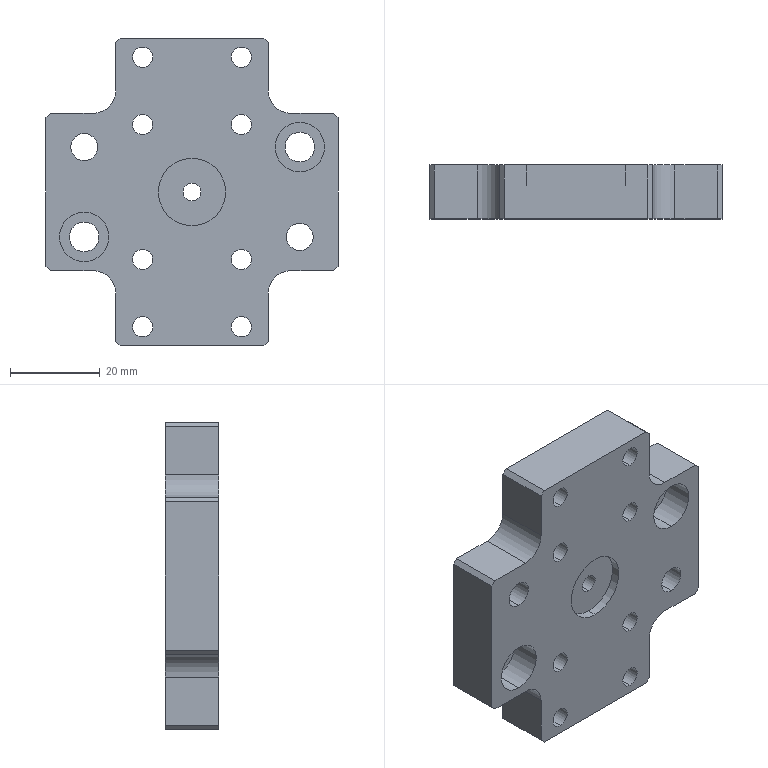Part | SolidWorks | features HoleWzd 3, ICE 2, Chamfer 1, Extrusion 1 | 1 solid | 85 faces | box 65 x 12 x 68.5 mm | volume 35580 mm3 | cylinder 52 | plane 33 | commonest cylinder face diameters 4.5 x16 8 x16 6 x4 6.6 x4 10 x4 11 x4